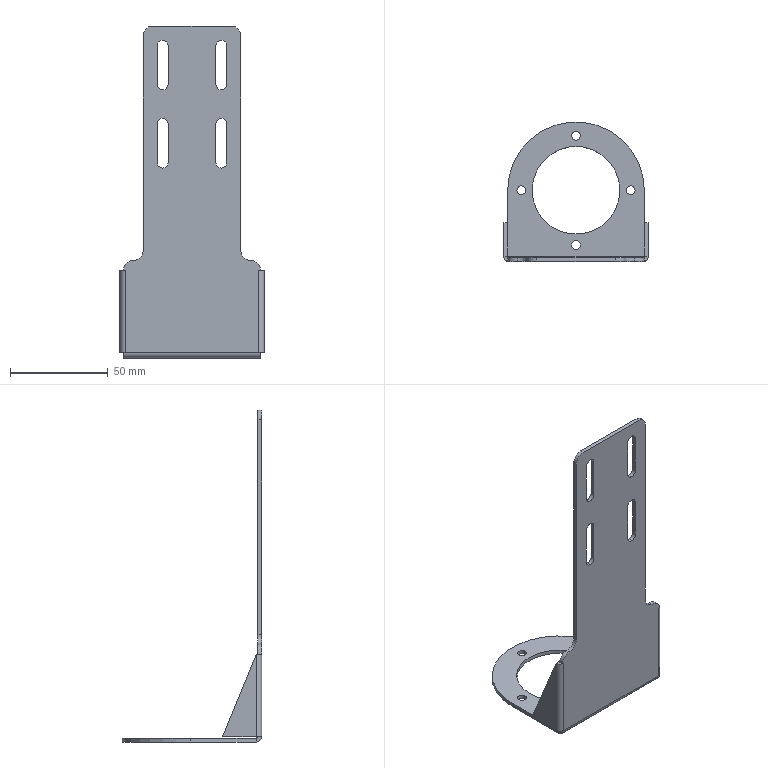Part | STEP file | 07-06 light source bracket (Default) | 1 solid | 70 faces | box 74 x 71.5 x 170 mm | volume 24970 mm3 | cylinder 35 | plane 35 | commonest cylinder face diameters 5.5 x12 4.5 x8 10 x6 1.473 x3 5.473 x3 45 x2